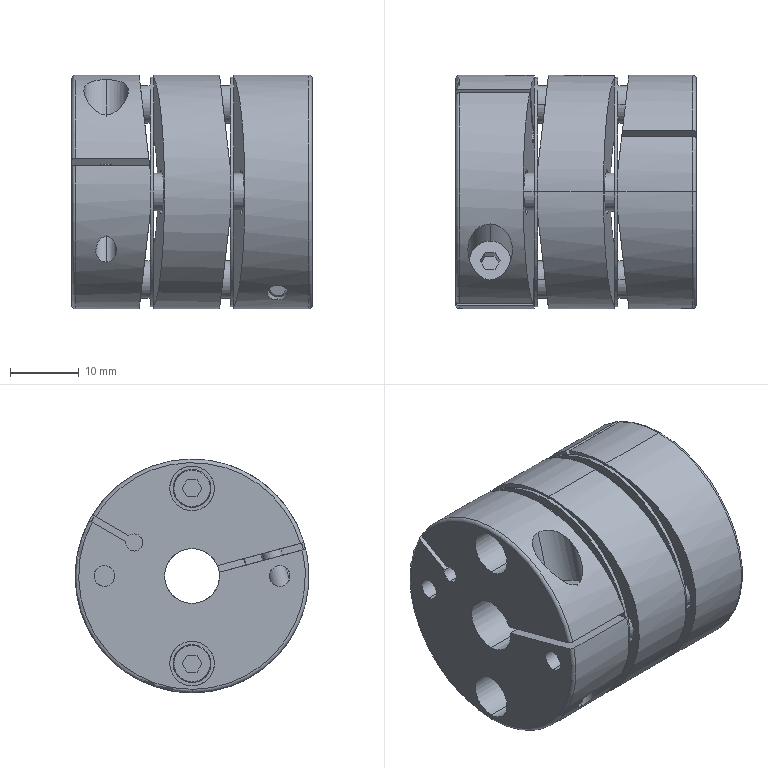Part | SolidWorks | features BaseBody 1 | 1 solid | 240 faces | box 35 x 34 x 34 mm | volume 23327 mm3 | plane 110 | cylinder 103 | cone 20 | torus 7 | commonest cylinder face diameters 3 x28 6.5 x20 5.5 x16 34 x9 2.5 x6 8 x6